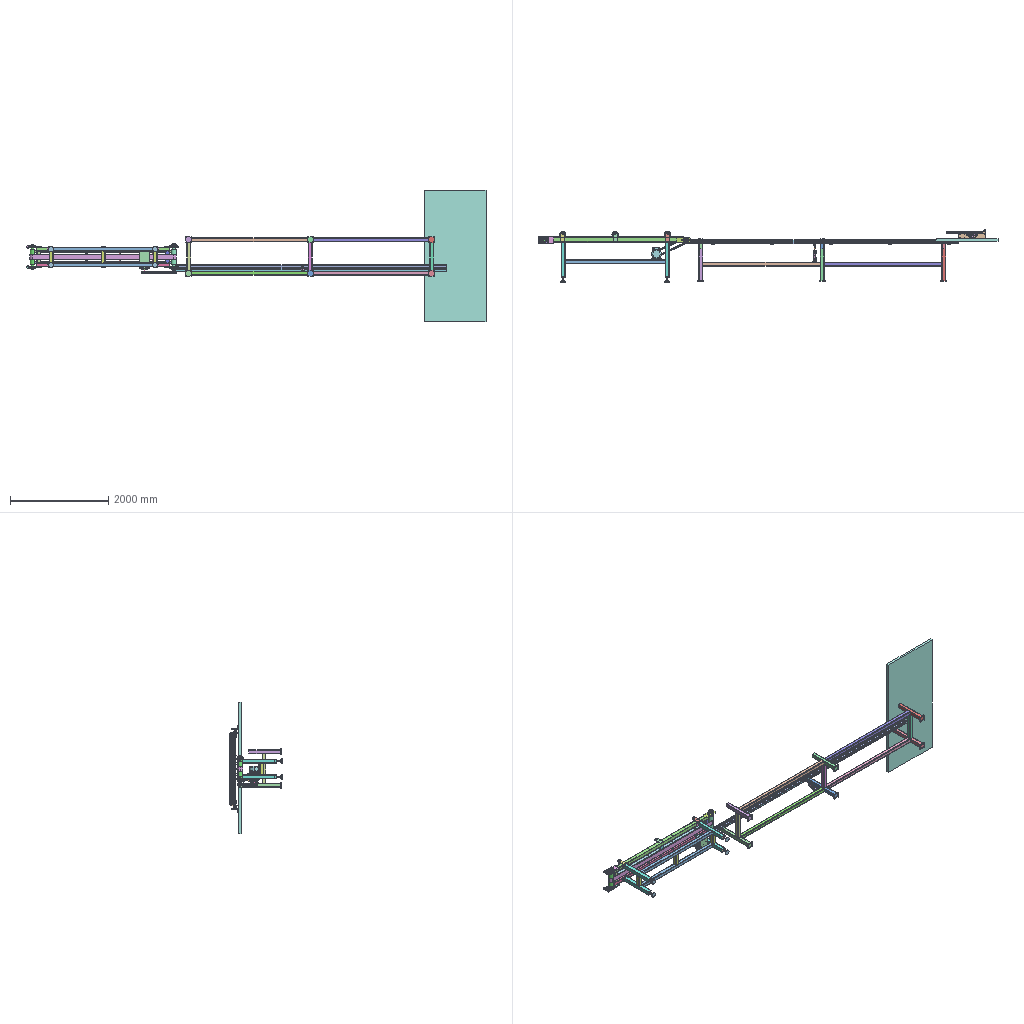Assembly | STEP file | 48 different items | 287 placed | box 9360 x 1063 x 2677 mm
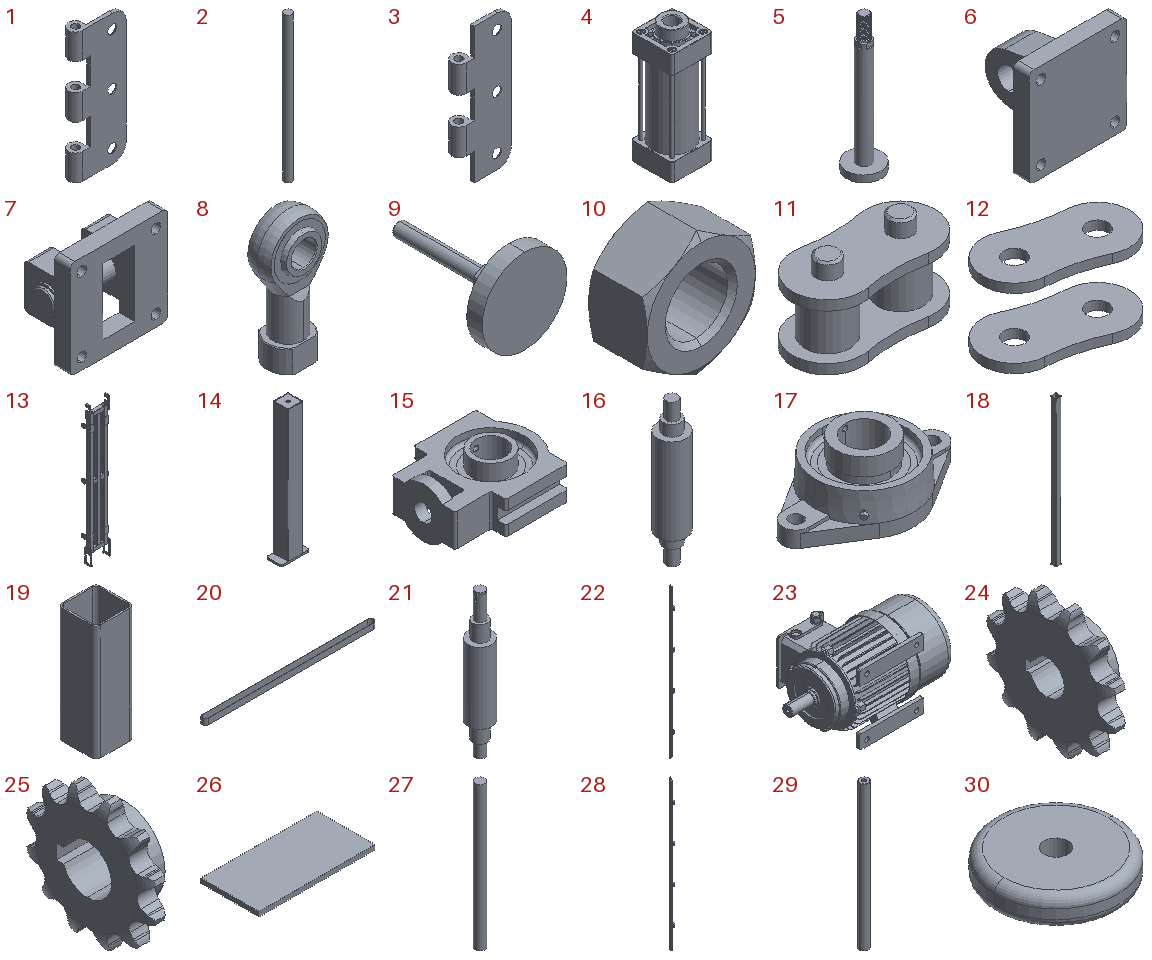Parts list (item | quantity | size | volume):
1 | x5 | 29 x 8 x 75 mm | 4670 mm3
2 | x5 | 4 x 4 x 75 mm | 942.478 mm3
3 | x5 | 29 x 8 x 75 mm | 4043 mm3
4 | x1 | 62 x 62 x 183 mm | 287709 mm3
5 | x1 | 50 x 50 x 197.5 mm | 73763 mm3
6 | x1 | 62 x 49 x 62 mm | 56958 mm3
7 | x1 | 62 x 34 x 62 mm | 54328 mm3
8 | x1 | 40 x 22 x 84 mm | 28902 mm3
9 | x4 | 100 x 148.5 x 100 mm | 234497 mm3
10 | x4 | 24 x 13 x 27.713 mm | 4447 mm3
11 | x96 | 49.53 x 24.13 x 33.5 mm | 14381 mm3
12 | x96 | 48.732 x 30.447 x 29.29 mm | 6239 mm3
13 | x1 | 442 x 225 x 3100 mm | 10604671 mm3
14 | x4 | 150 x 80 x 710 mm | 779802 mm3
15 | x2 | 146 x 124 x 67 mm | 474066 mm3
16 | x1 | 100 x 100 x 498 mm | 2727531 mm3
17 | x2 | 172 x 105 x 58.9 mm | 260417 mm3
18 | x2 | 80 x 80 x 2040 mm | 1795651 mm3
19 | x3 | 80 x 80 x 240 mm | 211253 mm3
20 | x1 | 2985 x 110 x 100 mm | 3039827 mm3
21 | x1 | 100 x 100 x 607 mm | 2954002 mm3
22 | x1 | 70 x 40 x 2839 mm | 801093 mm3
23 | x1 | 377 x 239.1 x 196 mm | 8664532 mm3
24 | x1 | 30.002 x 105.245 x 105.245 mm | 117979 mm3
25 | x1 | 30.002 x 105.245 x 105.245 mm | 111853 mm3
26 | x1 | 400 x 200 x 16 mm | 1280000 mm3
27 | x4 | 25 x 25 x 380 mm | 186532 mm3
28 | x1 | 70 x 40 x 2839 mm | 801093 mm3
29 | x3 | 25 x 25 x 400 mm | 193039 mm3
30 | x3 | 130 x 130 x 30 mm | 366544 mm3
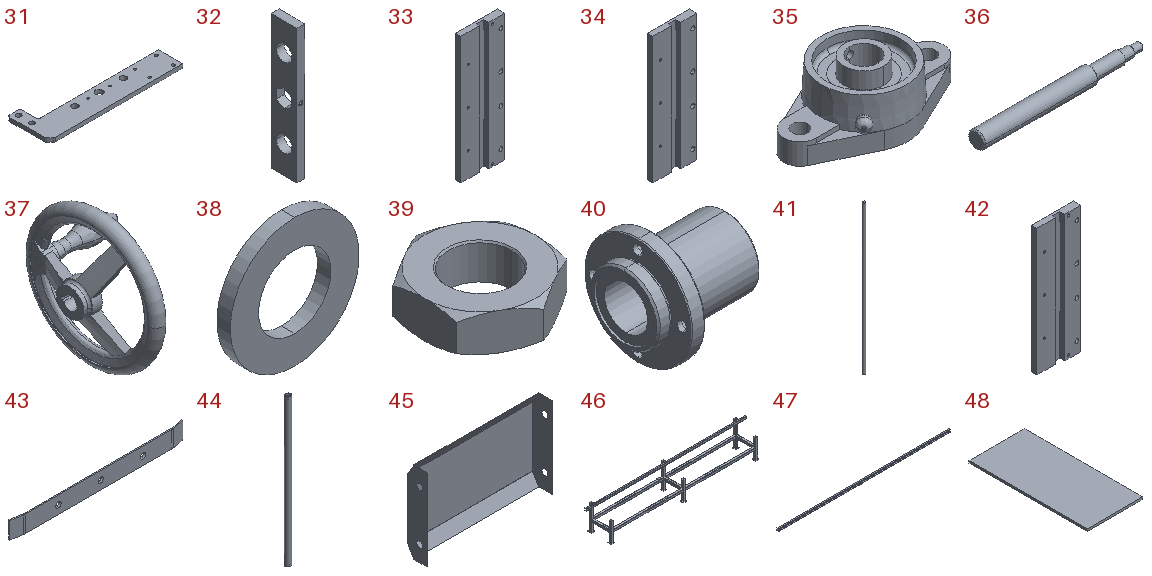31 | x2 | 549.959 x 175.002 x 16 mm | 892550 mm3
32 | x2 | 20 x 65 x 340 mm | 355958 mm3
33 | x1 | 112.747 x 19.5 x 340 mm | 560080 mm3
34 | x2 | 112.747 x 19.5 x 340 mm | 565839 mm3
35 | x2 | 113 x 62 x 37.3 mm | 69563 mm3
36 | x2 | 263 x 27 x 27 mm | 124305 mm3
37 | x2 | 117 x 160 x 160 mm | 172381 mm3
38 | x2 | 24 x 2.5 x 24 mm | 773.126 mm3
39 | x2 | 18 x 20.785 x 6 mm | 1162 mm3
40 | x4 | 59 x 62 x 62 mm | 56273 mm3
41 | x2 | 25 x 25 x 1510 mm | 741143 mm3
42 | x1 | 112.747 x 19.5 x 340 mm | 560080 mm3
43 | x4 | 409.088 x 8.069 x 40 mm | 48290 mm3
44 | x2 | 50 x 50 x 1450 mm | 1794980 mm3
45 | x1 | 504 x 80 x 327.138 mm | 217824 mm3
46 | x1 | 5500 x 803.417 x 860 mm | 20632149 mm3
47 | x1 | 5500 x 77.547 x 80 mm | 5816497 mm3
48 | x1 | 1260 x 2677 x 50 mm | 168683678 mm3
Placements (level | parent | child | x y z in mm | rotation matrix by rows):
1 | subassembly 2 | subassembly 3 | 1913.101 -145.588 4839.708 | 0 0 -1 1 0 0 0 -1 0
2 | subassembly 3 | subassembly 4 | -0.0 -0.0 -0.0 | 1 0 0 0 1 0 0 0 1
2 | subassembly 3 | subassembly 5 | -0.0 -0.0 -0.0 | 1 0 0 0 1 0 0 0 1
2 | subassembly 3 | subassembly 6 | -0.0 8.0 0.0 | 1 0 0 0 -1 0 0 0 -1
1 | subassembly 2 | subassembly 7 | -798.008 -343.197 4797.851 | 1 0 0 0 0.3552 0.9348 0 -0.9348 0.3552
2 | subassembly 7 | subassembly 8 | -24.166 -1.519 111.0 | 1 0 0 0 1 0 0 0 1
2 | subassembly 7 | subassembly 9 | -24.166 -1.519 171.359 | 0 1 0 -1 0 0 0 0 1
2 | subassembly 7 | subassembly 10 | -24.166 -1.519 -114.0 | 1 0 0 0 0 1 0 -1 0
2 | subassembly 7 | subassembly 11 | -24.166 -8.267 -165.761 | 1 0 0 0 0.3552 -0.9348 0 0.9348 0.3552
2 | subassembly 7 | subassembly 12 | -24.166 -1.519 139.359 | 0 -1 0 1 0 0 0 0 1
1 | subassembly 2 | subassembly 13 | 713.101 -145.588 4839.708 | 0 0 -1 1 0 0 0 -1 0
2 | subassembly 13 | subassembly 4 | -0.0 -0.0 -0.0 | 1 0 0 0 1 0 0 0 1
2 | subassembly 13 | subassembly 5 | -0.0 -0.0 -0.0 | 1 0 0 0 1 0 0 0 1
2 | subassembly 13 | subassembly 6 | 0.0 8.0 -0.0 | 1 0 0 0 -1 0 0 0 -1
1 | subassembly 2 | subassembly 14 | -486.899 -145.588 4839.708 | 0 0 -1 1 0 0 0 -1 0
2 | subassembly 14 | subassembly 4 | -0.0 -0.0 -0.0 | 1 0 0 0 1 0 0 0 1
2 | subassembly 14 | subassembly 5 | -0.0 -0.0 -0.0 | 1 0 0 0 1 0 0 0 1
2 | subassembly 14 | subassembly 6 | -0.0 8.0 -0.0 | 1 0 0 0 -1 0 0 0 -1
1 | subassembly 2 | subassembly 15 | -1686.899 -145.588 4839.708 | 0 0 -1 1 0 0 0 -1 0
2 | subassembly 15 | subassembly 4 | -0.0 -0.0 -0.0 | 1 0 0 0 1 0 0 0 1
2 | subassembly 15 | subassembly 5 | -0.0 -0.0 -0.0 | 1 0 0 0 1 0 0 0 1
2 | subassembly 15 | subassembly 6 | -0.0 8.0 -0.0 | 1 0 0 0 -1 0 0 0 -1
1 | subassembly 2 | subassembly 16 | -2886.899 -145.588 4839.708 | 0 0 -1 1 0 0 0 -1 0
2 | subassembly 16 | subassembly 4 | -0.0 -0.0 -0.0 | 1 0 0 0 1 0 0 0 1
2 | subassembly 16 | subassembly 5 | -0.0 -0.0 -0.0 | 1 0 0 0 1 0 0 0 1
2 | subassembly 16 | subassembly 6 | 0.0 8.0 -0.0 | 1 0 0 0 -1 0 0 0 -1
1 | subassembly 2 | subassembly 17 | -4879.399 -14.688 5075.587 | 0 0 1 0 1 0 -1 0 -0
2 | subassembly 17 | subassembly 18 | 160.0 -905.0 1060.0 | 0.8615 0 0.5077 0 1 0 -0.5077 0 0.8615
3 | subassembly 18 | subassembly 19 | 0.0 -0.0 -0.0 | 1 0 0 0 1 0 0 0 1
4 | subassembly 19 | subassembly 20 | -0.0 -0.0 -0.0 | 1 0 0 0 1 0 0 0 1
4 | subassembly 19 | subassembly 21 | -0.0 105.0 -0.0 | 1 0 0 0 -1 0 0 0 -1
2 | subassembly 17 | subassembly 22 | -160.0 -905.0 1060.0 | 0.8615 0 0.5077 0 1 0 -0.5077 0 0.8615
3 | subassembly 22 | subassembly 23 | 0.0 -0.0 -0.0 | 1 0 0 0 1 0 0 0 1
4 | subassembly 23 | subassembly 20 | -0.0 -0.0 -0.0 | 1 0 0 0 1 0 0 0 1
4 | subassembly 23 | subassembly 21 | -0.0 105.0 -0.0 | 1 0 0 0 -1 0 0 0 -1
2 | subassembly 17 | subassembly 24 | -160.0 -905.0 -1060.0 | 0.8615 0 0.5077 0 1 0 -0.5077 0 0.8615
3 | subassembly 24 | subassembly 25 | -0.0 -0.0 -0.0 | 1 0 0 0 1 0 0 0 1
4 | subassembly 25 | subassembly 20 | -0.0 -0.0 -0.0 | 1 0 0 0 1 0 0 0 1
4 | subassembly 25 | subassembly 21 | -0.0 105.0 0.0 | 1 0 0 0 -1 0 0 0 -1
2 | subassembly 17 | subassembly 26 | 160.0 -905.0 -1060.0 | 0.8615 0 0.5077 0 1 0 -0.5077 0 0.8615
3 | subassembly 26 | subassembly 27 | -0.0 -0.0 -0.0 | 1 0 0 0 1 0 0 0 1
4 | subassembly 27 | subassembly 20 | -0.0 -0.0 -0.0 | 1 0 0 0 1 0 0 0 1
4 | subassembly 27 | subassembly 21 | -0.0 105.0 0.0 | 1 0 0 0 -1 0 0 0 -1
2 | subassembly 17 | subassembly 28 | 312.447 -195.539 1133.667 | 0 0 1 -0.4303 0.9027 0 -0.9027 -0.4303 0
3 | subassembly 28 | subassembly 29 | -144.222 50.027 0.7292 | -1 0 0 0 1 0 0 0 -1
3 | subassembly 28 | subassembly 29 | -347.082 47.105 0.7292 | -0.9732 -0.2301 0 -0.2301 0.9732 0 0 0 -1
3 | subassembly 28 | subassembly 29 | -245.822 50.027 0.7292 | -1 0 0 0 1 0 0 0 -1
3 | subassembly 28 | subassembly 29 | -71.798 -48.111 0.7292 | 1 0 0 0 -1 0 0 0 -1
3 | subassembly 28 | subassembly 29 | -224.198 -48.111 0.7292 | 1 0 0 0 -1 0 0 0 -1
3 | subassembly 28 | subassembly 29 | -122.598 -48.111 0.7292 | 1 0 0 0 -1 0 0 0 -1
3 | subassembly 28 | subassembly 29 | 182.202 -48.111 0.7292 | 1 0 0 0 -1 0 0 0 -1
3 | subassembly 28 | subassembly 29 | -371.253 -30.96 0.7292 | 0.6734 -0.7392 0 -0.7392 -0.6734 0 0 0 -1
3 | subassembly 28 | subassembly 29 | 58.977 50.027 0.7292 | -1 0 0 0 1 0 0 0 -1
3 | subassembly 28 | subassembly 29 | -93.422 50.027 0.7292 | -1 0 0 0 1 0 0 0 -1
3 | subassembly 28 | subassembly 29 | -296.623 50.027 0.7292 | -1 0 0 0 1 0 0 0 -1
3 | subassembly 28 | subassembly 29 | 80.602 -48.111 0.7292 | 1 0 0 0 -1 0 0 0 -1
3 | subassembly 28 | subassembly 29 | -195.023 50.027 0.7292 | -1 0 0 0 1 0 0 0 -1
3 | subassembly 28 | subassembly 29 | -42.623 50.027 0.7292 | -1 0 0 0 1 0 0 0 -1
3 | subassembly 28 | subassembly 29 | 109.778 50.027 0.7292 | -1 0 0 0 1 0 0 0 -1
3 | subassembly 28 | subassembly 29 | 8.178 50.027 0.7292 | -1 0 0 0 1 0 0 0 -1
3 | subassembly 28 | subassembly 29 | -20.998 -48.111 0.7292 | 1 0 0 0 -1 0 0 0 -1
3 | subassembly 28 | subassembly 29 | 312.978 50.009 0.7292 | -1 0.001437 0 0.001437 1 0 0 0 -1
3 | subassembly 28 | subassembly 29 | -173.398 -48.111 0.7292 | 1 0 0 0 -1 0 0 0 -1
3 | subassembly 28 | subassembly 29 | 131.402 -48.111 0.7292 | 1 0 0 0 -1 0 0 0 -1
3 | subassembly 28 | subassembly 29 | 262.178 50.027 0.7292 | -1 0 0 0 1 0 0 0 -1
3 | subassembly 28 | subassembly 29 | -381.601 14.617 0.7292 | -0.2882 -0.9576 0 -0.9576 0.2882 0 0 0 -1
3 | subassembly 28 | subassembly 29 | 29.802 -48.111 0.7292 | 1 0 0 0 -1 0 0 0 -1
3 | subassembly 28 | subassembly 29 | 369.06 -13.065 0.7292 | 0.2959 0.9552 0 0.9552 -0.2959 0 0 0 -1
3 | subassembly 28 | subassembly 29 | 160.577 50.027 0.7292 | -1 0 0 0 1 0 0 0 -1
3 | subassembly 28 | subassembly 29 | 334.282 -45.281 0.7292 | 0.9749 0.2228 0 0.2228 -0.9749 0 0 0 -1
3 | subassembly 28 | subassembly 29 | 211.377 50.027 0.7292 | -1 0 0 0 1 0 0 0 -1
3 | subassembly 28 | subassembly 29 | 358.568 33.156 0.7292 | -0.6793 0.7338 0 0.7338 0.6793 0 0 0 -1
3 | subassembly 28 | subassembly 29 | 233.002 -48.111 0.7292 | 1 0 0 0 -1 0 0 0 -1
3 | subassembly 28 | subassembly 29 | -325.798 -48.084 0.7292 | 1 -0.002093 0 -0.002093 -1 0 0 0 -1
3 | subassembly 28 | subassembly 29 | 283.802 -48.111 0.7292 | 1 0 0 0 -1 0 0 0 -1
3 | subassembly 28 | subassembly 29 | -274.998 -48.111 0.7292 | 1 0 0 0 -1 0 0 0 -1
3 | subassembly 28 | subassembly 30 | -20.599 -44.953 26.679 | 0.9686 -0.2487 0 -0.2487 -0.9686 0 0 0 -1
3 | subassembly 28 | subassembly 30 | -195.422 46.869 26.679 | -0.9686 0.2487 0 0.2487 0.9686 0 0 0 -1
3 | subassembly 28 | subassembly 30 | -43.022 46.869 26.679 | -0.9686 0.2487 0 0.2487 0.9686 0 0 0 -1
3 | subassembly 28 | subassembly 30 | -223.799 -44.953 26.679 | 0.9686 -0.2487 0 -0.2487 -0.9686 0 0 0 -1
3 | subassembly 28 | subassembly 30 | 312.579 46.869 26.679 | -0.9686 0.2487 0 0.2487 0.9686 0 0 0 -1
3 | subassembly 28 | subassembly 30 | 335.491 -48.49 26.679 | 0.8797 0.4755 0 0.4755 -0.8797 0 0 0 -1
3 | subassembly 28 | subassembly 30 | 30.201 -44.953 26.679 | 0.9686 -0.2487 0 -0.2487 -0.9686 0 0 0 -1
3 | subassembly 28 | subassembly 30 | -348.317 50.31 26.679 | -0.8759 -0.4825 0 -0.4825 0.8759 0 0 0 -1
3 | subassembly 28 | subassembly 30 | -144.621 46.869 26.679 | -0.9686 0.2487 0 0.2487 0.9686 0 0 0 -1
3 | subassembly 28 | subassembly 30 | 160.179 46.869 26.679 | -0.9686 0.2487 0 0.2487 0.9686 0 0 0 -1
3 | subassembly 28 | subassembly 30 | -71.399 -44.953 26.679 | 0.9686 -0.2487 0 -0.2487 -0.9686 0 0 0 -1
3 | subassembly 28 | subassembly 30 | 233.401 -44.953 26.679 | 0.9686 -0.2487 0 -0.2487 -0.9686 0 0 0 -1
3 | subassembly 28 | subassembly 30 | -246.221 46.869 26.679 | -0.9686 0.2487 0 0.2487 0.9686 0 0 0 -1
3 | subassembly 28 | subassembly 30 | 109.379 46.869 26.679 | -0.9686 0.2487 0 0.2487 0.9686 0 0 0 -1
3 | subassembly 28 | subassembly 30 | -325.399 -44.953 26.679 | 0.9686 -0.2487 0 -0.2487 -0.9686 0 0 0 -1
3 | subassembly 28 | subassembly 30 | -297.022 46.869 26.679 | -0.9686 0.2487 0 0.2487 0.9686 0 0 0 -1
3 | subassembly 28 | subassembly 30 | -385.006 15.153 26.679 | -0.02005 -0.9998 0 -0.9998 0.02005 0 0 0 -1
3 | subassembly 28 | subassembly 30 | 182.601 -44.953 26.679 | 0.9686 -0.2487 0 -0.2487 -0.9686 0 0 0 -1
3 | subassembly 28 | subassembly 30 | -172.999 -44.953 26.679 | 0.9686 -0.2487 0 -0.2487 -0.9686 0 0 0 -1
3 | subassembly 28 | subassembly 30 | -274.599 -44.953 26.679 | 0.9686 -0.2487 0 -0.2487 -0.9686 0 0 0 -1
3 | subassembly 28 | subassembly 30 | 372.461 -13.629 26.679 | 0.02809 0.9996 0 0.9996 -0.02809 0 0 0 -1
3 | subassembly 28 | subassembly 30 | 81.001 -44.953 26.679 | 0.9686 -0.2487 0 -0.2487 -0.9686 0 0 0 -1
3 | subassembly 28 | subassembly 30 | 131.801 -44.953 26.679 | 0.9686 -0.2487 0 -0.2487 -0.9686 0 0 0 -1
3 | subassembly 28 | subassembly 30 | -93.822 46.869 26.679 | -0.9686 0.2487 0 0.2487 0.9686 0 0 0 -1
3 | subassembly 28 | subassembly 30 | -122.199 -44.953 26.679 | 0.9686 -0.2487 0 -0.2487 -0.9686 0 0 0 -1
3 | subassembly 28 | subassembly 30 | 284.201 -44.953 26.679 | 0.9686 -0.2487 0 -0.2487 -0.9686 0 0 0 -1
3 | subassembly 28 | subassembly 30 | 261.779 46.869 26.679 | -0.9686 0.2487 0 0.2487 0.9686 0 0 0 -1
3 | subassembly 28 | subassembly 30 | 360.756 35.819 26.679 | -0.8516 0.5241 0 0.5241 0.8516 0 0 0 -1
3 | subassembly 28 | subassembly 30 | -373.462 -33.606 26.679 | 0.8474 -0.5309 0 -0.5309 -0.8474 0 0 0 -1
3 | subassembly 28 | subassembly 30 | 210.978 46.869 26.679 | -0.9686 0.2487 0 0.2487 0.9686 0 0 0 -1
3 | subassembly 28 | subassembly 30 | 58.578 46.869 26.679 | -0.9686 0.2487 0 0.2487 0.9686 0 0 0 -1
3 | subassembly 28 | subassembly 30 | 7.779 46.869 26.679 | -0.9686 0.2487 0 0.2487 0.9686 0 0 0 -1
2 | subassembly 17 | subassembly 31 | 0.0 -40.0 -0.0 | 1 0 0 0 1 0 0 0 1
2 | subassembly 17 | subassembly 32 | -160.0 -90.0 1060.0 | 0 -1 0 0 0 -1 1 0 -0
2 | subassembly 17 | subassembly 32 | -160.0 -90.0 -1060.0 | 0 1 0 0 0 -1 -1 0 0
2 | subassembly 17 | subassembly 32 | 160.0 -90.0 -1060.0 | 0 1 0 0 0 -1 -1 0 0
2 | subassembly 17 | subassembly 32 | 160.0 -90.0 1060.0 | 0 -1 0 0 0 -1 1 0 -0
2 | subassembly 17 | subassembly 33 | -208.0 -50.0 -1438.143 | 0 0 -1 0 1 0 1 0 -0
2 | subassembly 17 | subassembly 33 | 208.0 -50.0 -1438.143 | 0 0 1 0 -1 0 1 0 -0
2 | subassembly 17 | subassembly 34 | -189.0 -50.0 -1438.143 | 0 0 1 0.7424 0.67 0 -0.67 0.7424 -0
2 | subassembly 17 | subassembly 35 | 216.0 -50.0 1436.75 | 0 0 1 0 -1 0 1 0 -0
2 | subassembly 17 | subassembly 35 | -216.0 -50.0 1436.75 | 0 0 -1 0 1 0 1 0 -0
2 | subassembly 17 | subassembly 36 | 160.0 -490.0 -0.0 | 1 0 0 0 1 0 0 0 1
2 | subassembly 17 | subassembly 36 | -160.0 -490.0 0.0 | 1 0 0 0 1 0 0 0 1
2 | subassembly 17 | subassembly 37 | -0.0 -490.0 -1060.0 | 0 0 1 0 1 0 -1 0 -0
2 | subassembly 17 | subassembly 37 | 0.0 -490.0 1060.0 | 0 0 1 0 1 0 -1 0 -0
2 | subassembly 17 | subassembly 37 | -0.0 -490.0 -0.0 | 0 0 1 0 1 0 -1 0 -0
2 | subassembly 17 | subassembly 38 | 0.5 -50.0 1436.75 | 0 0 -1 0 1 0 1 0 -0
2 | subassembly 17 | subassembly 39 | -218.5 -50.0 1436.75 | 0 0 1 0.05216 0.9986 0 -0.9986 0.05216 -0
2 | subassembly 17 | subassembly 40 | 110.0 12.0 -0.0 | 0 1 0 -1 0 0 0 0 1
2 | subassembly 17 | subassembly 41 | 127.5 -334.0 840.978 | -1 0 0 0 1 0 0 0 -1
2 | subassembly 17 | subassembly 42 | 313.176 -334.0 840.978 | -1 0 0 0 1 0 0 0 -1
2 | subassembly 17 | subassembly 43 | 313.176 -50.0 1436.75 | -1 0 0 0 -0.05216 0.9986 0 0.9986 0.05216
2 | subassembly 17 | subassembly 44 | 17.5 -434.0 840.978 | 1 0 0 0 0 -1 0 1 0
2 | subassembly 17 | subassembly 45 | 10.0 -25.0 1012.5 | 0 0 1 0.6978 0.7163 0 -0.7163 0.6978 0
2 | subassembly 17 | subassembly 45 | 10.0 -25.0 -1012.5 | 0 0 1 0.6978 0.7163 0 -0.7163 0.6978 0
2 | subassembly 17 | subassembly 45 | 10.0 -25.0 337.5 | 0 0 1 0.6978 0.7163 0 -0.7163 0.6978 0
2 | subassembly 17 | subassembly 45 | 10.0 -25.0 -337.5 | 0 0 1 0.6978 0.7163 0 -0.7163 0.6978 0
2 | subassembly 17 | subassembly 46 | -110.0 12.0 0.0 | 0 -1 0 -1 0 0 0 0 -1
2 | subassembly 17 | subassembly 47 | -0.0 70.0 0.0 | 0 0 1 0 1 0 -1 0 0
2 | subassembly 17 | subassembly 47 | -0.0 70.0 1068.406 | 0 0 1 0 1 0 -1 0 0
2 | subassembly 17 | subassembly 47 | -0.0 70.0 -1068.406 | 0 0 1 0 1 0 -1 0 0
2 | subassembly 17 | subassembly 48 | 0.0 70.0 0.0 | 0 0 -1 0 1 0 1 0 -0
2 | subassembly 17 | subassembly 48 | -0.0 70.0 -1068.406 | 0 0 -1 0 1 0 1 0 -0
2 | subassembly 17 | subassembly 48 | 0.0 70.0 1068.406 | 0 0 -1 0.1853 -0.9827 0 -0.9827 -0.1853 -0
1 | subassembly 2 | subassembly 49 | 2111.946 -1.1 5050.604 | 0 0 1 0 1 0 -1 0 -0
2 | subassembly 49 | subassembly 50 | 591.368 92.481 154.173 | 0 -1 0 0 0 -1 1 0 -0
3 | subassembly 50 | subassembly 29 | 283.802 -48.111 0.7292 | 1 0 0 0 -1 0 0 0 -1
3 | subassembly 50 | subassembly 29 | 358.568 33.156 0.7292 | -0.6793 0.7338 0 0.7338 0.6793 0 0 0 -1
3 | subassembly 50 | subassembly 29 | 182.202 -48.111 0.7292 | 1 0 0 0 -1 0 0 0 -1
3 | subassembly 50 | subassembly 29 | 80.602 -48.111 0.7292 | 1 0 0 0 -1 0 0 0 -1
3 | subassembly 50 | subassembly 29 | -144.222 50.027 0.7292 | -1 0 0 0 1 0 0 0 -1
3 | subassembly 50 | subassembly 29 | -42.623 50.027 0.7292 | -1 0 0 0 1 0 0 0 -1
3 | subassembly 50 | subassembly 29 | -224.198 -48.111 0.7292 | 1 0 0 0 -1 0 0 0 -1
3 | subassembly 50 | subassembly 29 | 334.282 -45.281 0.7292 | 0.9749 0.2228 0 0.2228 -0.9749 0 0 0 -1
3 | subassembly 50 | subassembly 29 | 312.978 50.009 0.7292 | -1 0.001437 0 0.001437 1 0 0 0 -1
3 | subassembly 50 | subassembly 29 | 58.977 50.027 0.7292 | -1 0 0 0 1 0 0 0 -1
3 | subassembly 50 | subassembly 29 | -381.601 14.617 0.7292 | -0.2882 -0.9576 0 -0.9576 0.2882 0 0 0 -1
3 | subassembly 50 | subassembly 29 | -173.398 -48.111 0.7292 | 1 0 0 0 -1 0 0 0 -1
3 | subassembly 50 | subassembly 29 | 369.06 -13.065 0.7292 | 0.2959 0.9552 0 0.9552 -0.2959 0 0 0 -1
3 | subassembly 50 | subassembly 29 | 131.402 -48.111 0.7292 | 1 0 0 0 -1 0 0 0 -1
3 | subassembly 50 | subassembly 29 | 8.178 50.027 0.7292 | -1 0 0 0 1 0 0 0 -1
3 | subassembly 50 | subassembly 29 | 29.802 -48.111 0.7292 | 1 0 0 0 -1 0 0 0 -1
3 | subassembly 50 | subassembly 29 | -195.023 50.027 0.7292 | -1 0 0 0 1 0 0 0 -1
3 | subassembly 50 | subassembly 29 | -245.822 50.027 0.7292 | -1 0 0 0 1 0 0 0 -1
3 | subassembly 50 | subassembly 29 | -347.082 47.105 0.7292 | -0.9732 -0.2301 0 -0.2301 0.9732 0 0 0 -1
3 | subassembly 50 | subassembly 29 | -274.998 -48.111 0.7292 | 1 0 0 0 -1 0 0 0 -1
3 | subassembly 50 | subassembly 29 | -296.623 50.027 0.7292 | -1 0 0 0 1 0 0 0 -1
3 | subassembly 50 | subassembly 29 | -20.998 -48.111 0.7292 | 1 0 0 0 -1 0 0 0 -1
3 | subassembly 50 | subassembly 29 | 262.178 50.027 0.7292 | -1 0 0 0 1 0 0 0 -1
3 | subassembly 50 | subassembly 29 | 211.377 50.027 0.7292 | -1 0 0 0 1 0 0 0 -1
3 | subassembly 50 | subassembly 29 | -122.598 -48.111 0.7292 | 1 0 0 0 -1 0 0 0 -1
3 | subassembly 50 | subassembly 29 | 233.002 -48.111 0.7292 | 1 0 0 0 -1 0 0 0 -1
3 | subassembly 50 | subassembly 29 | 160.577 50.027 0.7292 | -1 0 0 0 1 0 0 0 -1
3 | subassembly 50 | subassembly 29 | -93.422 50.027 0.7292 | -1 0 0 0 1 0 0 0 -1
3 | subassembly 50 | subassembly 29 | 109.778 50.027 0.7292 | -1 0 0 0 1 0 0 0 -1
3 | subassembly 50 | subassembly 29 | -325.798 -48.084 0.7292 | 1 -0.002093 0 -0.002093 -1 0 0 0 -1
3 | subassembly 50 | subassembly 29 | -71.798 -48.111 0.7292 | 1 0 0 0 -1 0 0 0 -1
3 | subassembly 50 | subassembly 29 | -371.253 -30.96 0.7292 | 0.6734 -0.7392 0 -0.7392 -0.6734 0 0 0 -1
3 | subassembly 50 | subassembly 30 | 7.779 46.869 26.679 | -0.9686 0.2487 0 0.2487 0.9686 0 0 0 -1
3 | subassembly 50 | subassembly 30 | 284.201 -44.953 26.679 | 0.9686 -0.2487 0 -0.2487 -0.9686 0 0 0 -1
3 | subassembly 50 | subassembly 30 | 160.179 46.869 26.679 | -0.9686 0.2487 0 0.2487 0.9686 0 0 0 -1
3 | subassembly 50 | subassembly 30 | -373.462 -33.606 26.679 | 0.8474 -0.5309 0 -0.5309 -0.8474 0 0 0 -1
3 | subassembly 50 | subassembly 30 | 210.978 46.869 26.679 | -0.9686 0.2487 0 0.2487 0.9686 0 0 0 -1
3 | subassembly 50 | subassembly 30 | -297.022 46.869 26.679 | -0.9686 0.2487 0 0.2487 0.9686 0 0 0 -1
3 | subassembly 50 | subassembly 30 | -223.799 -44.953 26.679 | 0.9686 -0.2487 0 -0.2487 -0.9686 0 0 0 -1
3 | subassembly 50 | subassembly 30 | -195.422 46.869 26.679 | -0.9686 0.2487 0 0.2487 0.9686 0 0 0 -1
3 | subassembly 50 | subassembly 30 | 58.578 46.869 26.679 | -0.9686 0.2487 0 0.2487 0.9686 0 0 0 -1
3 | subassembly 50 | subassembly 30 | -385.006 15.153 26.679 | -0.02005 -0.9998 0 -0.9998 0.02005 0 0 0 -1
3 | subassembly 50 | subassembly 30 | 30.201 -44.953 26.679 | 0.9686 -0.2487 0 -0.2487 -0.9686 0 0 0 -1
3 | subassembly 50 | subassembly 30 | 261.779 46.869 26.679 | -0.9686 0.2487 0 0.2487 0.9686 0 0 0 -1
3 | subassembly 50 | subassembly 30 | 372.461 -13.629 26.679 | 0.02809 0.9996 0 0.9996 -0.02809 0 0 0 -1
3 | subassembly 50 | subassembly 30 | -325.399 -44.953 26.679 | 0.9686 -0.2487 0 -0.2487 -0.9686 0 0 0 -1
3 | subassembly 50 | subassembly 30 | 131.801 -44.953 26.679 | 0.9686 -0.2487 0 -0.2487 -0.9686 0 0 0 -1
3 | subassembly 50 | subassembly 30 | 109.379 46.869 26.679 | -0.9686 0.2487 0 0.2487 0.9686 0 0 0 -1
3 | subassembly 50 | subassembly 30 | -144.621 46.869 26.679 | -0.9686 0.2487 0 0.2487 0.9686 0 0 0 -1
3 | subassembly 50 | subassembly 30 | -172.999 -44.953 26.679 | 0.9686 -0.2487 0 -0.2487 -0.9686 0 0 0 -1
3 | subassembly 50 | subassembly 30 | 335.491 -48.49 26.679 | 0.8797 0.4755 0 0.4755 -0.8797 0 0 0 -1
3 | subassembly 50 | subassembly 30 | 81.001 -44.953 26.679 | 0.9686 -0.2487 0 -0.2487 -0.9686 0 0 0 -1
3 | subassembly 50 | subassembly 30 | 312.579 46.869 26.679 | -0.9686 0.2487 0 0.2487 0.9686 0 0 0 -1
3 | subassembly 50 | subassembly 30 | -122.199 -44.953 26.679 | 0.9686 -0.2487 0 -0.2487 -0.9686 0 0 0 -1
3 | subassembly 50 | subassembly 30 | -348.317 50.31 26.679 | -0.8759 -0.4825 0 -0.4825 0.8759 0 0 0 -1
3 | subassembly 50 | subassembly 30 | 360.756 35.819 26.679 | -0.8516 0.5241 0 0.5241 0.8516 0 0 0 -1
3 | subassembly 50 | subassembly 30 | 182.601 -44.953 26.679 | 0.9686 -0.2487 0 -0.2487 -0.9686 0 0 0 -1
3 | subassembly 50 | subassembly 30 | -71.399 -44.953 26.679 | 0.9686 -0.2487 0 -0.2487 -0.9686 0 0 0 -1
3 | subassembly 50 | subassembly 30 | -20.599 -44.953 26.679 | 0.9686 -0.2487 0 -0.2487 -0.9686 0 0 0 -1
3 | subassembly 50 | subassembly 30 | -246.221 46.869 26.679 | -0.9686 0.2487 0 0.2487 0.9686 0 0 0 -1
3 | subassembly 50 | subassembly 30 | 233.401 -44.953 26.679 | 0.9686 -0.2487 0 -0.2487 -0.9686 0 0 0 -1
3 | subassembly 50 | subassembly 30 | -93.822 46.869 26.679 | -0.9686 0.2487 0 0.2487 0.9686 0 0 0 -1
3 | subassembly 50 | subassembly 30 | -274.599 -44.953 26.679 | 0.9686 -0.2487 0 -0.2487 -0.9686 0 0 0 -1
3 | subassembly 50 | subassembly 30 | -43.022 46.869 26.679 | -0.9686 0.2487 0 0.2487 0.9686 0 0 0 -1
2 | subassembly 49 | subassembly 51 | -631.368 91.023 154.173 | 0 1 0 0 0 1 1 0 0
3 | subassembly 51 | subassembly 29 | -274.998 -48.111 0.7292 | 1 0 0 0 -1 0 0 0 -1
3 | subassembly 51 | subassembly 29 | 312.978 50.009 0.7292 | -1 0.001437 0 0.001437 1 0 0 0 -1
3 | subassembly 51 | subassembly 29 | 160.577 50.027 0.7292 | -1 0 0 0 1 0 0 0 -1
3 | subassembly 51 | subassembly 29 | -144.222 50.027 0.7292 | -1 0 0 0 1 0 0 0 -1
3 | subassembly 51 | subassembly 29 | -20.998 -48.111 0.7292 | 1 0 0 0 -1 0 0 0 -1
3 | subassembly 51 | subassembly 29 | -245.822 50.027 0.7292 | -1 0 0 0 1 0 0 0 -1
3 | subassembly 51 | subassembly 29 | -42.623 50.027 0.7292 | -1 0 0 0 1 0 0 0 -1
3 | subassembly 51 | subassembly 29 | 182.202 -48.111 0.7292 | 1 0 0 0 -1 0 0 0 -1
3 | subassembly 51 | subassembly 29 | -347.082 47.105 0.7292 | -0.9732 -0.2301 0 -0.2301 0.9732 0 0 0 -1
3 | subassembly 51 | subassembly 29 | 211.377 50.027 0.7292 | -1 0 0 0 1 0 0 0 -1
3 | subassembly 51 | subassembly 29 | -371.253 -30.96 0.7292 | 0.6734 -0.7392 0 -0.7392 -0.6734 0 0 0 -1
3 | subassembly 51 | subassembly 29 | -71.798 -48.111 0.7292 | 1 0 0 0 -1 0 0 0 -1
3 | subassembly 51 | subassembly 29 | 109.778 50.027 0.7292 | -1 0 0 0 1 0 0 0 -1
3 | subassembly 51 | subassembly 29 | -173.398 -48.111 0.7292 | 1 0 0 0 -1 0 0 0 -1
3 | subassembly 51 | subassembly 29 | 58.977 50.027 0.7292 | -1 0 0 0 1 0 0 0 -1
3 | subassembly 51 | subassembly 29 | 233.002 -48.111 0.7292 | 1 0 0 0 -1 0 0 0 -1
3 | subassembly 51 | subassembly 29 | -381.601 14.617 0.7292 | -0.2882 -0.9576 0 -0.9576 0.2882 0 0 0 -1
3 | subassembly 51 | subassembly 29 | -195.023 50.027 0.7292 | -1 0 0 0 1 0 0 0 -1
3 | subassembly 51 | subassembly 29 | 8.178 50.027 0.7292 | -1 0 0 0 1 0 0 0 -1
3 | subassembly 51 | subassembly 29 | 334.282 -45.281 0.7292 | 0.9749 0.2228 0 0.2228 -0.9749 0 0 0 -1
3 | subassembly 51 | subassembly 29 | -93.422 50.027 0.7292 | -1 0 0 0 1 0 0 0 -1
3 | subassembly 51 | subassembly 29 | -296.623 50.027 0.7292 | -1 0 0 0 1 0 0 0 -1
3 | subassembly 51 | subassembly 29 | 80.602 -48.111 0.7292 | 1 0 0 0 -1 0 0 0 -1
3 | subassembly 51 | subassembly 29 | -122.598 -48.111 0.7292 | 1 0 0 0 -1 0 0 0 -1
3 | subassembly 51 | subassembly 29 | 283.802 -48.111 0.7292 | 1 0 0 0 -1 0 0 0 -1
3 | subassembly 51 | subassembly 29 | 131.402 -48.111 0.7292 | 1 0 0 0 -1 0 0 0 -1
3 | subassembly 51 | subassembly 29 | -224.198 -48.111 0.7292 | 1 0 0 0 -1 0 0 0 -1
3 | subassembly 51 | subassembly 29 | 29.802 -48.111 0.7292 | 1 0 0 0 -1 0 0 0 -1
3 | subassembly 51 | subassembly 29 | 358.568 33.156 0.7292 | -0.6793 0.7338 0 0.7338 0.6793 0 0 0 -1
3 | subassembly 51 | subassembly 29 | 369.06 -13.065 0.7292 | 0.2959 0.9552 0 0.9552 -0.2959 0 0 0 -1
3 | subassembly 51 | subassembly 29 | 262.178 50.027 0.7292 | -1 0 0 0 1 0 0 0 -1
3 | subassembly 51 | subassembly 29 | -325.798 -48.084 0.7292 | 1 -0.002093 0 -0.002093 -1 0 0 0 -1
3 | subassembly 51 | subassembly 30 | -297.022 46.869 26.679 | -0.9686 0.2487 0 0.2487 0.9686 0 0 0 -1
3 | subassembly 51 | subassembly 30 | 261.779 46.869 26.679 | -0.9686 0.2487 0 0.2487 0.9686 0 0 0 -1
3 | subassembly 51 | subassembly 30 | -325.399 -44.953 26.679 | 0.9686 -0.2487 0 -0.2487 -0.9686 0 0 0 -1
3 | subassembly 51 | subassembly 30 | 160.179 46.869 26.679 | -0.9686 0.2487 0 0.2487 0.9686 0 0 0 -1
3 | subassembly 51 | subassembly 30 | 182.601 -44.953 26.679 | 0.9686 -0.2487 0 -0.2487 -0.9686 0 0 0 -1
3 | subassembly 51 | subassembly 30 | 7.779 46.869 26.679 | -0.9686 0.2487 0 0.2487 0.9686 0 0 0 -1
3 | subassembly 51 | subassembly 30 | -274.599 -44.953 26.679 | 0.9686 -0.2487 0 -0.2487 -0.9686 0 0 0 -1
3 | subassembly 51 | subassembly 30 | -246.221 46.869 26.679 | -0.9686 0.2487 0 0.2487 0.9686 0 0 0 -1
3 | subassembly 51 | subassembly 30 | -195.422 46.869 26.679 | -0.9686 0.2487 0 0.2487 0.9686 0 0 0 -1
3 | subassembly 51 | subassembly 30 | -43.022 46.869 26.679 | -0.9686 0.2487 0 0.2487 0.9686 0 0 0 -1
3 | subassembly 51 | subassembly 30 | 81.001 -44.953 26.679 | 0.9686 -0.2487 0 -0.2487 -0.9686 0 0 0 -1
3 | subassembly 51 | subassembly 30 | -144.621 46.869 26.679 | -0.9686 0.2487 0 0.2487 0.9686 0 0 0 -1
3 | subassembly 51 | subassembly 30 | -385.006 15.153 26.679 | -0.02005 -0.9998 0 -0.9998 0.02005 0 0 0 -1
3 | subassembly 51 | subassembly 30 | -172.999 -44.953 26.679 | 0.9686 -0.2487 0 -0.2487 -0.9686 0 0 0 -1
3 | subassembly 51 | subassembly 30 | -20.599 -44.953 26.679 | 0.9686 -0.2487 0 -0.2487 -0.9686 0 0 0 -1
3 | subassembly 51 | subassembly 30 | 58.578 46.869 26.679 | -0.9686 0.2487 0 0.2487 0.9686 0 0 0 -1
3 | subassembly 51 | subassembly 30 | 372.461 -13.629 26.679 | 0.02809 0.9996 0 0.9996 -0.02809 0 0 0 -1
3 | subassembly 51 | subassembly 30 | 30.201 -44.953 26.679 | 0.9686 -0.2487 0 -0.2487 -0.9686 0 0 0 -1
3 | subassembly 51 | subassembly 30 | -223.799 -44.953 26.679 | 0.9686 -0.2487 0 -0.2487 -0.9686 0 0 0 -1
3 | subassembly 51 | subassembly 30 | -93.822 46.869 26.679 | -0.9686 0.2487 0 0.2487 0.9686 0 0 0 -1
3 | subassembly 51 | subassembly 30 | -348.317 50.31 26.679 | -0.8759 -0.4825 0 -0.4825 0.8759 0 0 0 -1
3 | subassembly 51 | subassembly 30 | 109.379 46.869 26.679 | -0.9686 0.2487 0 0.2487 0.9686 0 0 0 -1
3 | subassembly 51 | subassembly 30 | 360.756 35.819 26.679 | -0.8516 0.5241 0 0.5241 0.8516 0 0 0 -1
3 | subassembly 51 | subassembly 30 | 131.801 -44.953 26.679 | 0.9686 -0.2487 0 -0.2487 -0.9686 0 0 0 -1
3 | subassembly 51 | subassembly 30 | -122.199 -44.953 26.679 | 0.9686 -0.2487 0 -0.2487 -0.9686 0 0 0 -1
3 | subassembly 51 | subassembly 30 | 312.579 46.869 26.679 | -0.9686 0.2487 0 0.2487 0.9686 0 0 0 -1
3 | subassembly 51 | subassembly 30 | 284.201 -44.953 26.679 | 0.9686 -0.2487 0 -0.2487 -0.9686 0 0 0 -1
3 | subassembly 51 | subassembly 30 | -71.399 -44.953 26.679 | 0.9686 -0.2487 0 -0.2487 -0.9686 0 0 0 -1
3 | subassembly 51 | subassembly 30 | 233.401 -44.953 26.679 | 0.9686 -0.2487 0 -0.2487 -0.9686 0 0 0 -1
3 | subassembly 51 | subassembly 30 | 210.978 46.869 26.679 | -0.9686 0.2487 0 0.2487 0.9686 0 0 0 -1
3 | subassembly 51 | subassembly 30 | -373.462 -33.606 26.679 | 0.8474 -0.5309 0 -0.5309 -0.8474 0 0 0 -1
3 | subassembly 51 | subassembly 30 | 335.491 -48.49 26.679 | 0.8797 0.4755 0 0.4755 -0.8797 0 0 0 -1
2 | subassembly 49 | subassembly 52 | -763.5 -57.998 7.109 | 0 0 1 0 1 0 -1 0 -0
2 | subassembly 49 | subassembly 52 | 707.5 -57.998 7.109 | 0 0 1 0 1 0 -1 0 -0
2 | subassembly 49 | subassembly 53 | 655.687 36.502 107.109 | 1 0 0 0 1 0 0 0 1
2 | subassembly 49 | subassembly 53 | -695.687 36.502 447.11 | -1 0 0 0 1 0 0 0 -1
2 | subassembly 49 | subassembly 54 | 605.687 98.252 277.11 | 1 0 0 0 1 0 0 0 1
2 | subassembly 49 | subassembly 55 | -645.687 78.752 277.11 | -1 0 0 0 -1 0 0 0 1
2 | subassembly 49 | subassembly 55 | 605.687 78.752 277.11 | 1 0 0 0 -1 0 0 0 -1
2 | subassembly 49 | subassembly 56 | 723.5 36.502 277.11 | 0 0 1 0 1 0 -1 0 0
2 | subassembly 49 | subassembly 56 | -763.5 36.502 277.11 | 0 0 -1 0 1 0 1 0 0
2 | subassembly 49 | subassembly 57 | 575.474 36.502 277.11 | 1 0 0 0 -0.9954 0.0957 0 -0.0957 -0.9954
2 | subassembly 49 | subassembly 57 | -615.474 36.502 277.11 | -1 0 0 0 -0.9954 -0.0957 0 -0.0957 0.9954
2 | subassembly 49 | subassembly 58 | -800.8 36.502 277.11 | -1 0 0 0 -0.9954 -0.0957 0 -0.0957 0.9954
2 | subassembly 49 | subassembly 58 | 760.8 36.502 277.11 | 1 0 0 0 -0.9954 0.0957 0 -0.0957 -0.9954
2 | subassembly 49 | subassembly 59 | 791.944 36.502 277.11 | 0 -1 0 1 0 0 0 0 1
2 | subassembly 49 | subassembly 59 | -831.944 36.502 277.11 | 0 1 0 1 0 0 0 0 -1
2 | subassembly 49 | subassembly 60 | -823.3 36.502 277.11 | 0 0 -1 -0.312 0.9501 0 0.9501 0.312 0
2 | subassembly 49 | subassembly 60 | 789.3 36.502 277.11 | 0 0 -1 -0.312 0.9501 0 0.9501 0.312 -0
2 | subassembly 49 | subassembly 61 | -721.687 36.502 377.11 | 1 0 0 0 -1 0 0 0 -1
2 | subassembly 49 | subassembly 61 | 681.687 36.502 177.109 | -1 0 0 0 1 0 0 0 -1
2 | subassembly 49 | subassembly 61 | 681.687 36.502 377.11 | -1 0 0 0 1 0 0 0 -1
2 | subassembly 49 | subassembly 61 | -721.687 36.502 177.109 | 1 0 0 0 -1 0 0 0 -1
2 | subassembly 49 | subassembly 62 | -20.0 36.502 377.11 | 0 0 1 0.9224 -0.3863 0 0.3863 0.9224 -0
2 | subassembly 49 | subassembly 62 | -20.0 36.502 177.109 | 0 0 1 -0.8608 -0.509 0 0.509 -0.8608 -0
2 | subassembly 49 | subassembly 63 | -645.687 98.252 277.11 | -1 0 0 0 1 0 0 0 -1
2 | subassembly 49 | subassembly 64 | -632.94 93.502 277.11 | 0 0 1 0 1 0 -1 0 -0
2 | subassembly 49 | subassembly 64 | 552.94 93.502 277.11 | 0 0 1 0 1 0 -1 0 0
2 | subassembly 49 | subassembly 64 | -592.94 83.502 277.11 | 0 0 -1 0 -1 0 -1 0 0
2 | subassembly 49 | subassembly 64 | 592.94 83.502 277.11 | 0 0 -1 0 -1 0 -1 0 -0
2 | subassembly 49 | subassembly 65 | -20.0 65.002 526.11 | 0 0 1 0 1 0 -1 0 -0
2 | subassembly 49 | subassembly 65 | -20.0 120.002 526.11 | 0 0 1 -0.05702 0.9984 0 -0.9984 -0.05702 -0
2 | subassembly 49 | subassembly 66 | -57.105 85.752 157.109 | 1 0 0 0 1 0 0 0 1
1 | subassembly 2 | subassembly 67 | -3141.107 -891.088 4745.0 | 1 0 0 0 0 1 0 -1 0
1 | subassembly 2 | subassembly 68 | -649.399 -96.088 4839.708 | 1 0 0 0 1 0 0 0 1
1 | subassembly 2 | subassembly 69 | -3141.107 -61.088 4745.0 | 1 0 0 0 0 1 0 -1 0